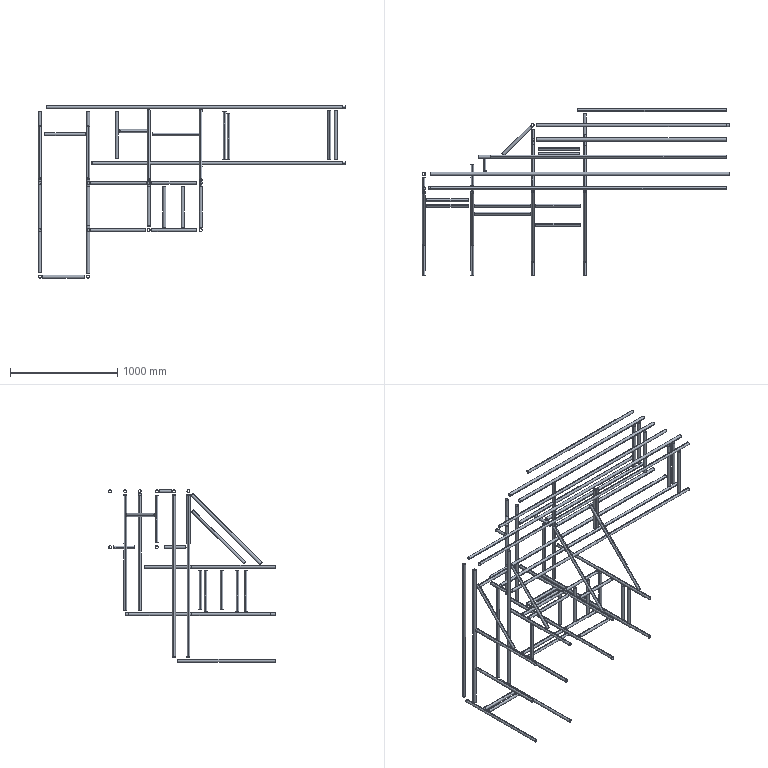Part | STEP file | CAIDA A V3_Predeterminado<Como mecanizada> | 68 solids | 408 faces | box 2864 x 1554 x 1609 mm | volume 6177747 mm3 | cylinder 273 | plane 135 | commonest cylinder face diameters 28.6 x137 26.2 x136